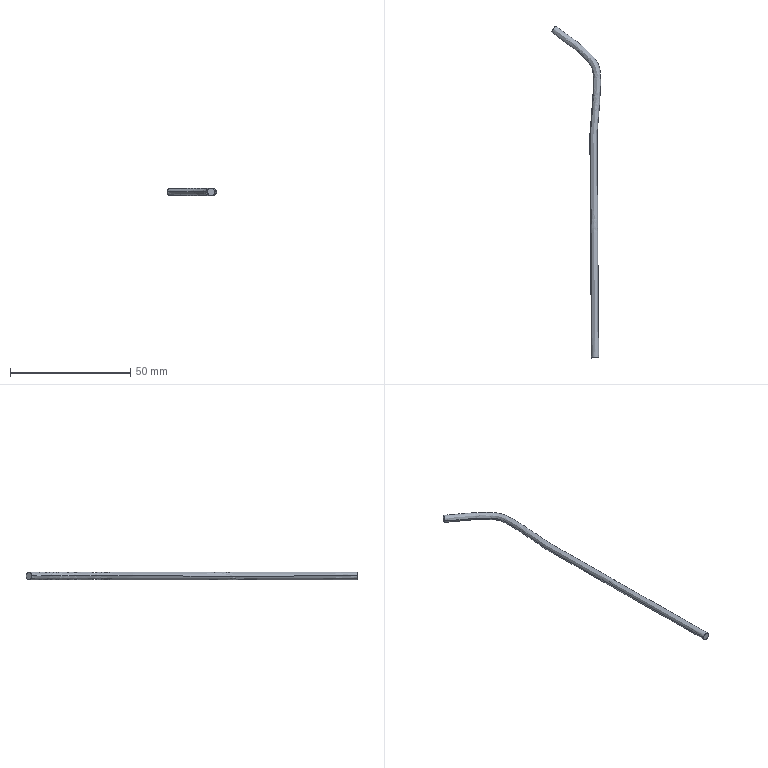Part | NX | features BREP 1 | 1 solid | 4 faces | box 20.548 x 138.141 x 3 mm | volume 1002 mm3 | plane 2 | spline 2
STEP:
#1=CARTESIAN_POINT('',(61.593,-31.891,217.465));
#2=VERTEX_POINT('',#1);
#3=CARTESIAN_POINT('',(64.593,-31.865,217.465));
#4=VERTEX_POINT('',#3);
#5=CARTESIAN_POINT('',(61.593,-31.891,217.465));
#6=CARTESIAN_POINT('',(61.593,-31.891,217.819));
#7=CARTESIAN_POINT('',(61.861,-31.889,218.592));
#8=CARTESIAN_POINT('',(63.093,-31.878,219.152));
#9=CARTESIAN_POINT('',(64.325,-31.867,218.592));
#10=CARTESIAN_POINT('',(64.593,-31.865,217.819));
#11=CARTESIAN_POINT('',(64.593,-31.865,217.465));
#12=B_SPLINE_CURVE_WITH_KNOTS('',3,(#5,#6,#7,#8,#9,#10,#11),.UNSPECIFIED.,.F.,.F.,(4,1,1,1,4),(0.,0.25,0.5,0.75,1.),.UNSPECIFIED.);
#13=EDGE_CURVE('',#2,#4,#12,.T.);
#14=ORIENTED_EDGE('',*,*,#13,.F.);
#15=CARTESIAN_POINT('',(64.593,-31.865,217.465));
#16=CARTESIAN_POINT('',(64.593,-31.865,217.111));
#17=CARTESIAN_POINT('',(64.325,-31.867,216.338));
#18=CARTESIAN_POINT('',(63.093,-31.878,215.778));
#19=CARTESIAN_POINT('',(61.861,-31.889,216.338));
#20=CARTESIAN_POINT('',(61.593,-31.891,217.111));
#21=CARTESIAN_POINT('',(61.593,-31.891,217.465));
#22=B_SPLINE_CURVE_WITH_KNOTS('',3,(#15,#16,#17,#18,#19,#20,#21),.UNSPECIFIED.,.F.,.F.,(4,1,1,1,4),(0.,0.25,0.5,0.75,1.),.QUASI_UNIFORM_KNOTS.);
#23=EDGE_CURVE('',#4,#2,#22,.T.);
#24=ORIENTED_EDGE('',*,*,#23,.F.);
#25=EDGE_LOOP('',(#14,#24));
#26=FACE_BOUND('',#25,.T.);
#27=CARTESIAN_POINT('',(61.593,-31.891,217.465));
#28=DIRECTION('',(0.008906,-1.,0.000000006));
#29=DIRECTION('',(0.,0.000000006,1.));
#30=AXIS2_PLACEMENT_3D('',#27,#28,#29);
#31=PLANE('',#30);
#32=ADVANCED_FACE('',(#26),#31,.T.);
#33=CARTESIAN_POINT('',(44.894,103.809,217.465));
#34=VERTEX_POINT('',#33);
#35=CARTESIAN_POINT('',(44.894,103.809,217.465));
#36=CARTESIAN_POINT('',(46.116,102.935,217.465));
#37=CARTESIAN_POINT('',(48.783,100.951,217.465));
#38=CARTESIAN_POINT('',(52.514,98.365,217.465));
#39=CARTESIAN_POINT('',(55.95,95.618,217.465));
#40=CARTESIAN_POINT('',(58.626,93.056,217.465));
#41=CARTESIAN_POINT('',(60.651,90.876,217.465));
#42=CARTESIAN_POINT('',(61.601,89.557,217.465));
#43=CARTESIAN_POINT('',(61.978,88.512,217.465));
#44=CARTESIAN_POINT('',(62.247,87.211,217.465));
#45=CARTESIAN_POINT('',(62.413,85.422,217.465));
#46=CARTESIAN_POINT('',(62.458,83.217,217.465));
#47=CARTESIAN_POINT('',(62.394,80.239,217.465));
#48=CARTESIAN_POINT('',(62.18,76.415,217.465));
#49=CARTESIAN_POINT('',(61.919,72.728,217.465));
#50=CARTESIAN_POINT('',(61.677,69.609,217.465));
#51=CARTESIAN_POINT('',(61.506,67.528,217.465));
#52=CARTESIAN_POINT('',(61.373,66.009,217.465));
#53=CARTESIAN_POINT('',(61.249,64.63,217.465));
#54=CARTESIAN_POINT('',(61.139,63.519,217.465));
#55=CARTESIAN_POINT('',(61.066,62.809,217.465));
#56=CARTESIAN_POINT('',(60.906,61.459,217.465));
#57=CARTESIAN_POINT('',(60.942,60.335,217.465));
#58=CARTESIAN_POINT('',(60.935,58.917,217.465));
#59=CARTESIAN_POINT('',(60.945,58.217,217.465));
#60=CARTESIAN_POINT('',(60.956,56.671,217.465));
#61=CARTESIAN_POINT('',(60.969,55.141,217.465));
#62=CARTESIAN_POINT('',(60.987,53.132,217.465));
#63=CARTESIAN_POINT('',(61.019,49.703,217.465));
#64=CARTESIAN_POINT('',(61.062,44.953,217.465));
#65=CARTESIAN_POINT('',(61.109,39.145,217.465));
#66=CARTESIAN_POINT('',(61.145,34.01,217.465));
#67=CARTESIAN_POINT('',(61.182,27.92,217.465));
#68=CARTESIAN_POINT('',(61.224,20.363,217.465));
#69=CARTESIAN_POINT('',(61.274,12.258,217.465));
#70=CARTESIAN_POINT('',(61.333,4.336,217.465));
#71=CARTESIAN_POINT('',(61.401,-4.1,217.465));
#72=CARTESIAN_POINT('',(61.473,-13.387,217.465));
#73=CARTESIAN_POINT('',(61.529,-22.629,217.465));
#74=CARTESIAN_POINT('',(61.566,-28.804,217.465));
#75=CARTESIAN_POINT('',(61.593,-31.891,217.465));
#76=B_SPLINE_CURVE_WITH_KNOTS('',3,(#35,#36,#37,#38,#39,#40,#41,#42,#43,#44,#45,#46,#47,#48,#49,#50,#51,#52,#53,#54,#55,#56,#57,#58,#59,#60,#61,#62,#63,#64,#65,#66,#67,#68,#69,#70,#71,#72,#73,#74,#75),.UNSPECIFIED.,.F.,.F.,(4,1,1,1,1,1,1,1,1,1,1,1,1,1,1,1,1,1,1,1,1,1,1,1,1,1,1,1,1,1,1,1,1,1,1,1,1,1,4),(0.,0.03125,0.0625,0.09375,0.125,0.1406,0.1562,0.1641,0.1719,0.1875,0.2031,0.2188,0.25,0.2812,0.2969,0.3125,0.3281,0.3438,0.3477,0.3516,0.3594,0.3672,0.375,0.3906,0.3984,0.4062,0.4219,0.4375,0.4688,0.5,0.5312,0.5625,0.625,0.6875,0.75,0.8125,0.875,0.9375,1.),.UNSPECIFIED.);
#77=EDGE_CURVE('',#34,#2,#76,.T.);
#78=ORIENTED_EDGE('',*,*,#77,.T.);
#79=ORIENTED_EDGE('',*,*,#13,.T.);
#80=CARTESIAN_POINT('',(46.638,106.249,217.465));
#81=VERTEX_POINT('',#80);
#82=CARTESIAN_POINT('',(64.593,-31.865,217.465));
#83=CARTESIAN_POINT('',(64.565,-28.783,217.465));
#84=CARTESIAN_POINT('',(64.529,-22.614,217.465));
#85=CARTESIAN_POINT('',(64.473,-13.365,217.465));
#86=CARTESIAN_POINT('',(64.401,-4.075,217.465));
#87=CARTESIAN_POINT('',(64.333,4.36,217.465));
#88=CARTESIAN_POINT('',(64.274,12.277,217.465));
#89=CARTESIAN_POINT('',(64.224,20.379,217.465));
#90=CARTESIAN_POINT('',(64.182,27.937,217.465));
#91=CARTESIAN_POINT('',(64.145,34.03,217.465));
#92=CARTESIAN_POINT('',(64.109,39.166,217.465));
#93=CARTESIAN_POINT('',(64.062,44.977,217.465));
#94=CARTESIAN_POINT('',(64.019,49.728,217.465));
#95=CARTESIAN_POINT('',(63.987,53.159,217.465));
#96=CARTESIAN_POINT('',(63.968,55.168,217.465));
#97=CARTESIAN_POINT('',(63.956,56.695,217.465));
#98=CARTESIAN_POINT('',(63.944,58.236,217.465));
#99=CARTESIAN_POINT('',(63.939,58.934,217.465));
#100=CARTESIAN_POINT('',(63.935,60.159,217.465));
#101=CARTESIAN_POINT('',(63.935,60.903,217.465));
#102=CARTESIAN_POINT('',(63.94,61.42,217.465));
#103=CARTESIAN_POINT('',(63.949,61.631,217.465));
#104=CARTESIAN_POINT('',(63.977,61.879,217.465));
#105=CARTESIAN_POINT('',(64.028,62.324,217.465));
#106=CARTESIAN_POINT('',(64.074,62.744,217.465));
#107=CARTESIAN_POINT('',(64.124,63.223,217.465));
#108=CARTESIAN_POINT('',(64.198,63.97,217.465));
#109=CARTESIAN_POINT('',(64.277,64.818,217.465));
#110=CARTESIAN_POINT('',(64.383,65.993,217.465));
#111=CARTESIAN_POINT('',(64.495,67.275,217.465));
#112=CARTESIAN_POINT('',(64.667,69.371,217.465));
#113=CARTESIAN_POINT('',(64.91,72.507,217.465));
#114=CARTESIAN_POINT('',(65.173,76.219,217.465));
#115=CARTESIAN_POINT('',(65.393,80.1,217.465));
#116=CARTESIAN_POINT('',(65.457,83.207,217.465));
#117=CARTESIAN_POINT('',(65.414,85.566,217.465));
#118=CARTESIAN_POINT('',(65.224,87.598,217.465));
#119=CARTESIAN_POINT('',(64.899,89.256,217.465));
#120=CARTESIAN_POINT('',(64.241,91.075,217.465));
#121=CARTESIAN_POINT('',(62.896,92.872,217.465));
#122=CARTESIAN_POINT('',(61.283,94.603,217.465));
#123=CARTESIAN_POINT('',(59.649,96.225,217.465));
#124=CARTESIAN_POINT('',(57.318,98.371,217.465));
#125=CARTESIAN_POINT('',(54.277,100.792,217.465));
#126=CARTESIAN_POINT('',(50.495,103.415,217.465));
#127=CARTESIAN_POINT('',(47.924,105.33,217.465));
#128=CARTESIAN_POINT('',(46.638,106.249,217.465));
#129=B_SPLINE_CURVE_WITH_KNOTS('',3,(#82,#83,#84,#85,#86,#87,#88,#89,#90,#91,#92,#93,#94,#95,#96,#97,#98,#99,#100,#101,#102,#103,#104,#105,#106,#107,#108,#109,#110,#111,#112,#113,#114,#115,#116,#117,#118,#119,#120,#121,#122,#123,#124,#125,#126,#127,#128),.UNSPECIFIED.,.F.,.F.,(4,1,1,1,1,1,1,1,1,1,1,1,1,1,1,1,1,1,1,1,1,1,1,1,1,1,1,1,1,1,1,1,1,1,1,1,1,1,1,1,1,1,1,1,4),(0.,0.0625,0.125,0.1875,0.25,0.3125,0.375,0.4375,0.4688,0.5,0.5312,0.5625,0.5781,0.5938,0.6016,0.6094,0.625,0.6328,0.6367,0.6406,0.6426,0.6445,0.6465,0.6484,0.6523,0.6562,0.6641,0.6719,0.6875,0.7031,0.7188,0.75,0.7812,0.7969,0.8125,0.8281,0.8359,0.8438,0.8594,0.875,0.8906,0.9062,0.9375,0.9688,1.),.UNSPECIFIED.);
#130=EDGE_CURVE('',#81,#4,#129,.F.);
#131=ORIENTED_EDGE('',*,*,#130,.F.);
#132=CARTESIAN_POINT('',(44.894,103.809,217.465));
#133=CARTESIAN_POINT('',(44.894,103.809,217.819));
#134=CARTESIAN_POINT('',(45.05,104.027,218.592));
#135=CARTESIAN_POINT('',(45.766,105.029,219.152));
#136=CARTESIAN_POINT('',(46.482,106.031,218.592));
#137=CARTESIAN_POINT('',(46.638,106.249,217.819));
#138=CARTESIAN_POINT('',(46.638,106.249,217.465));
#139=B_SPLINE_CURVE_WITH_KNOTS('',3,(#132,#133,#134,#135,#136,#137,#138),.UNSPECIFIED.,.F.,.F.,(4,1,1,1,4),(0.,0.25,0.5,0.75,1.),.UNSPECIFIED.);
#140=EDGE_CURVE('',#34,#81,#139,.T.);
#141=ORIENTED_EDGE('',*,*,#140,.F.);
#142=EDGE_LOOP('',(#78,#79,#131,#141));
#143=FACE_BOUND('',#142,.T.);
#144=CARTESIAN_POINT('',(64.593,-31.865,217.465));
#145=CARTESIAN_POINT('',(64.593,-31.865,217.819));
#146=CARTESIAN_POINT('',(64.325,-31.867,218.592));
#147=CARTESIAN_POINT('',(63.093,-31.878,219.152));
#148=CARTESIAN_POINT('',(61.861,-31.889,218.592));
#149=CARTESIAN_POINT('',(61.593,-31.891,217.819));
#150=CARTESIAN_POINT('',(61.593,-31.891,217.465));
#151=CARTESIAN_POINT('',(64.563,-28.51,217.465));
#152=CARTESIAN_POINT('',(64.563,-28.51,217.819));
#153=CARTESIAN_POINT('',(64.295,-28.512,218.592));
#154=CARTESIAN_POINT('',(63.063,-28.52,219.152));
#155=CARTESIAN_POINT('',(61.831,-28.529,218.592));
#156=CARTESIAN_POINT('',(61.563,-28.53,217.819));
#157=CARTESIAN_POINT('',(61.563,-28.53,217.465));
#158=CARTESIAN_POINT('',(64.534,-23.475,217.465));
#159=CARTESIAN_POINT('',(64.534,-23.475,217.819));
#160=CARTESIAN_POINT('',(64.266,-23.477,218.592));
#161=CARTESIAN_POINT('',(63.034,-23.483,219.152));
#162=CARTESIAN_POINT('',(61.802,-23.49,218.592));
#163=CARTESIAN_POINT('',(61.534,-23.491,217.819));
#164=CARTESIAN_POINT('',(61.534,-23.491,217.465));
#165=CARTESIAN_POINT('',(64.494,-16.759,217.465));
#166=CARTESIAN_POINT('',(64.494,-16.759,217.819));
#167=CARTESIAN_POINT('',(64.226,-16.76,218.592));
#168=CARTESIAN_POINT('',(62.994,-16.768,219.152));
#169=CARTESIAN_POINT('',(61.762,-16.776,218.592));
#170=CARTESIAN_POINT('',(61.494,-16.778,217.819));
#171=CARTESIAN_POINT('',(61.494,-16.778,217.465));
#172=CARTESIAN_POINT('',(64.458,-11.449,217.465));
#173=CARTESIAN_POINT('',(64.458,-11.449,217.819));
#174=CARTESIAN_POINT('',(64.189,-11.451,218.592));
#175=CARTESIAN_POINT('',(62.958,-11.46,219.152));
#176=CARTESIAN_POINT('',(61.726,-11.469,218.592));
#177=CARTESIAN_POINT('',(61.458,-11.471,217.819));
#178=CARTESIAN_POINT('',(61.458,-11.471,217.465));
#179=CARTESIAN_POINT('',(64.415,-5.882,217.465));
#180=CARTESIAN_POINT('',(64.415,-5.882,217.819));
#181=CARTESIAN_POINT('',(64.147,-5.884,218.592));
#182=CARTESIAN_POINT('',(62.915,-5.894,219.152));
#183=CARTESIAN_POINT('',(61.683,-5.904,218.592));
#184=CARTESIAN_POINT('',(61.415,-5.906,217.819));
#185=CARTESIAN_POINT('',(61.415,-5.906,217.465));
#186=CARTESIAN_POINT('',(64.356,1.522,217.465));
#187=CARTESIAN_POINT('',(64.356,1.522,217.819));
#188=CARTESIAN_POINT('',(64.087,1.52,218.592));
#189=CARTESIAN_POINT('',(62.856,1.51,219.152));
#190=CARTESIAN_POINT('',(61.624,1.5,218.592));
#191=CARTESIAN_POINT('',(61.356,1.498,217.819));
#192=CARTESIAN_POINT('',(61.356,1.498,217.465));
#193=CARTESIAN_POINT('',(64.289,9.937,217.465));
#194=CARTESIAN_POINT('',(64.289,9.937,217.819));
#195=CARTESIAN_POINT('',(64.021,9.936,218.592));
#196=CARTESIAN_POINT('',(62.789,9.927,219.152));
#197=CARTESIAN_POINT('',(61.557,9.918,218.592));
#198=CARTESIAN_POINT('',(61.289,9.917,217.819));
#199=CARTESIAN_POINT('',(61.289,9.917,217.465));
#200=CARTESIAN_POINT('',(64.236,18.351,217.465));
#201=CARTESIAN_POINT('',(64.236,18.351,217.819));
#202=CARTESIAN_POINT('',(63.968,18.35,218.592));
#203=CARTESIAN_POINT('',(62.736,18.343,219.152));
#204=CARTESIAN_POINT('',(61.504,18.336,218.592));
#205=CARTESIAN_POINT('',(61.236,18.334,217.819));
#206=CARTESIAN_POINT('',(61.236,18.334,217.465));
#207=CARTESIAN_POINT('',(64.194,25.757,217.465));
#208=CARTESIAN_POINT('',(64.194,25.757,217.819));
#209=CARTESIAN_POINT('',(63.926,25.756,218.592));
#210=CARTESIAN_POINT('',(62.694,25.749,219.152));
#211=CARTESIAN_POINT('',(61.462,25.742,218.592));
#212=CARTESIAN_POINT('',(61.194,25.741,217.819));
#213=CARTESIAN_POINT('',(61.194,25.741,217.465));
#214=CARTESIAN_POINT('',(64.166,30.569,217.465));
#215=CARTESIAN_POINT('',(64.166,30.569,217.819));
#216=CARTESIAN_POINT('',(63.898,30.568,218.592));
#217=CARTESIAN_POINT('',(62.666,30.56,219.152));
#218=CARTESIAN_POINT('',(61.435,30.553,218.592));
#219=CARTESIAN_POINT('',(61.167,30.552,217.819));
#220=CARTESIAN_POINT('',(61.167,30.552,217.465));
#221=CARTESIAN_POINT('',(64.142,34.39,217.465));
#222=CARTESIAN_POINT('',(64.142,34.39,217.819));
#223=CARTESIAN_POINT('',(63.874,34.388,218.592));
#224=CARTESIAN_POINT('',(62.642,34.38,219.152));
#225=CARTESIAN_POINT('',(61.411,34.372,218.592));
#226=CARTESIAN_POINT('',(61.142,34.371,217.819));
#227=CARTESIAN_POINT('',(61.142,34.371,217.465));
#228=CARTESIAN_POINT('',(64.114,38.442,217.465));
#229=CARTESIAN_POINT('',(64.114,38.442,217.819));
#230=CARTESIAN_POINT('',(63.846,38.44,218.592));
#231=CARTESIAN_POINT('',(62.614,38.431,219.152));
#232=CARTESIAN_POINT('',(61.383,38.422,218.592));
#233=CARTESIAN_POINT('',(61.114,38.42,217.819));
#234=CARTESIAN_POINT('',(61.114,38.42,217.465));
#235=CARTESIAN_POINT('',(64.069,44.22,217.465));
#236=CARTESIAN_POINT('',(64.069,44.22,217.819));
#237=CARTESIAN_POINT('',(63.801,44.218,218.592));
#238=CARTESIAN_POINT('',(62.569,44.209,219.152));
#239=CARTESIAN_POINT('',(61.337,44.199,218.592));
#240=CARTESIAN_POINT('',(61.069,44.197,217.819));
#241=CARTESIAN_POINT('',(61.069,44.197,217.465));
#242=CARTESIAN_POINT('',(64.006,51.151,217.465));
#243=CARTESIAN_POINT('',(64.006,51.151,217.819));
#244=CARTESIAN_POINT('',(63.738,51.149,218.592));
#245=CARTESIAN_POINT('',(62.506,51.138,219.152));
#246=CARTESIAN_POINT('',(61.275,51.127,218.592));
#247=CARTESIAN_POINT('',(61.006,51.125,217.819));
#248=CARTESIAN_POINT('',(61.006,51.125,217.465));
#249=CARTESIAN_POINT('',(63.965,55.427,217.465));
#250=CARTESIAN_POINT('',(63.965,55.427,217.819));
#251=CARTESIAN_POINT('',(63.697,55.425,218.592));
#252=CARTESIAN_POINT('',(62.465,55.413,219.152));
#253=CARTESIAN_POINT('',(61.233,55.401,218.592));
#254=CARTESIAN_POINT('',(60.965,55.398,217.819));
#255=CARTESIAN_POINT('',(60.965,55.398,217.465));
#256=CARTESIAN_POINT('',(63.946,57.988,217.465));
#257=CARTESIAN_POINT('',(63.946,57.988,217.819));
#258=CARTESIAN_POINT('',(63.678,57.986,218.592));
#259=CARTESIAN_POINT('',(62.446,57.978,219.152));
#260=CARTESIAN_POINT('',(61.214,57.969,218.592));
#261=CARTESIAN_POINT('',(60.946,57.968,217.819));
#262=CARTESIAN_POINT('',(60.946,57.968,217.465));
#263=CARTESIAN_POINT('',(63.941,58.709,217.465));
#264=CARTESIAN_POINT('',(63.941,58.709,217.819));
#265=CARTESIAN_POINT('',(63.673,58.708,218.592));
#266=CARTESIAN_POINT('',(62.441,58.702,219.152));
#267=CARTESIAN_POINT('',(61.21,58.696,218.592));
#268=CARTESIAN_POINT('',(60.941,58.694,217.819));
#269=CARTESIAN_POINT('',(60.941,58.694,217.465));
#270=CARTESIAN_POINT('',(63.937,59.434,217.465));
#271=CARTESIAN_POINT('',(63.937,59.434,217.819));
#272=CARTESIAN_POINT('',(63.669,59.433,218.592));
#273=CARTESIAN_POINT('',(62.437,59.429,219.152));
#274=CARTESIAN_POINT('',(61.206,59.425,218.592));
#275=CARTESIAN_POINT('',(60.937,59.424,217.819));
#276=CARTESIAN_POINT('',(60.937,59.424,217.465));
#277=CARTESIAN_POINT('',(63.934,60.323,217.465));
#278=CARTESIAN_POINT('',(63.934,60.323,217.819));
#279=CARTESIAN_POINT('',(63.666,60.322,218.592));
#280=CARTESIAN_POINT('',(62.434,60.317,219.152));
#281=CARTESIAN_POINT('',(61.202,60.312,218.592));
#282=CARTESIAN_POINT('',(60.934,60.311,217.819));
#283=CARTESIAN_POINT('',(60.934,60.311,217.465));
#284=CARTESIAN_POINT('',(63.936,60.979,217.465));
#285=CARTESIAN_POINT('',(63.936,60.979,217.819));
#286=CARTESIAN_POINT('',(63.668,60.981,218.592));
#287=CARTESIAN_POINT('',(62.436,60.99,219.152));
#288=CARTESIAN_POINT('',(61.204,60.999,218.592));
#289=CARTESIAN_POINT('',(60.936,61.001,217.819));
#290=CARTESIAN_POINT('',(60.936,61.001,217.465));
#291=CARTESIAN_POINT('',(63.939,61.327,217.465));
#292=CARTESIAN_POINT('',(63.939,61.327,217.819));
#293=CARTESIAN_POINT('',(63.671,61.329,218.592));
#294=CARTESIAN_POINT('',(62.439,61.34,219.152));
#295=CARTESIAN_POINT('',(61.208,61.35,218.592));
#296=CARTESIAN_POINT('',(60.939,61.353,217.819));
#297=CARTESIAN_POINT('',(60.939,61.353,217.465));
#298=CARTESIAN_POINT('',(63.945,61.554,217.465));
#299=CARTESIAN_POINT('',(63.945,61.554,217.819));
#300=CARTESIAN_POINT('',(63.677,61.565,218.592));
#301=CARTESIAN_POINT('',(62.446,61.616,219.152));
#302=CARTESIAN_POINT('',(61.214,61.667,218.592));
#303=CARTESIAN_POINT('',(60.946,61.678,217.819));
#304=CARTESIAN_POINT('',(60.946,61.678,217.465));
#305=CARTESIAN_POINT('',(63.953,61.659,217.465));
#306=CARTESIAN_POINT('',(63.953,61.659,217.819));
#307=CARTESIAN_POINT('',(63.686,61.687,218.592));
#308=CARTESIAN_POINT('',(62.46,61.816,219.152));
#309=CARTESIAN_POINT('',(61.235,61.944,218.592));
#310=CARTESIAN_POINT('',(60.968,61.972,217.819));
#311=CARTESIAN_POINT('',(60.968,61.972,217.465));
#312=CARTESIAN_POINT('',(63.974,61.85,217.465));
#313=CARTESIAN_POINT('',(63.974,61.85,217.819));
#314=CARTESIAN_POINT('',(63.707,61.881,218.592));
#315=CARTESIAN_POINT('',(62.484,62.025,219.152));
#316=CARTESIAN_POINT('',(61.261,62.169,218.592));
#317=CARTESIAN_POINT('',(60.995,62.201,217.819));
#318=CARTESIAN_POINT('',(60.995,62.201,217.465));
#319=CARTESIAN_POINT('',(64.006,62.133,217.465));
#320=CARTESIAN_POINT('',(64.006,62.133,217.819));
#321=CARTESIAN_POINT('',(63.74,62.164,218.592));
#322=CARTESIAN_POINT('',(62.517,62.304,219.152));
#323=CARTESIAN_POINT('',(61.293,62.445,218.592));
#324=CARTESIAN_POINT('',(61.027,62.476,217.819));
#325=CARTESIAN_POINT('',(61.027,62.476,217.465));
#326=CARTESIAN_POINT('',(64.039,62.423,217.465));
#327=CARTESIAN_POINT('',(64.039,62.423,217.819));
#328=CARTESIAN_POINT('',(63.773,62.452,218.592));
#329=CARTESIAN_POINT('',(62.548,62.587,219.152));
#330=CARTESIAN_POINT('',(61.324,62.721,218.592));
#331=CARTESIAN_POINT('',(61.057,62.751,217.819));
#332=CARTESIAN_POINT('',(61.057,62.751,217.465));
#333=CARTESIAN_POINT('',(64.136,63.316,217.465));
#334=CARTESIAN_POINT('',(64.136,63.316,217.819));
#335=CARTESIAN_POINT('',(63.869,63.342,218.592));
#336=CARTESIAN_POINT('',(62.643,63.463,219.152));
#337=CARTESIAN_POINT('',(61.417,63.584,218.592));
#338=CARTESIAN_POINT('',(61.15,63.611,217.819));
#339=CARTESIAN_POINT('',(61.15,63.611,217.465));
#340=CARTESIAN_POINT('',(64.273,64.758,217.465));
#341=CARTESIAN_POINT('',(64.273,64.758,217.819));
#342=CARTESIAN_POINT('',(64.006,64.782,218.592));
#343=CARTESIAN_POINT('',(62.78,64.896,219.152));
#344=CARTESIAN_POINT('',(61.553,65.009,218.592));
#345=CARTESIAN_POINT('',(61.286,65.033,217.819));
#346=CARTESIAN_POINT('',(61.286,65.033,217.465));
#347=CARTESIAN_POINT('',(64.411,66.305,217.465));
#348=CARTESIAN_POINT('',(64.411,66.305,217.819));
#349=CARTESIAN_POINT('',(64.144,66.329,218.592));
#350=CARTESIAN_POINT('',(62.917,66.438,219.152));
#351=CARTESIAN_POINT('',(61.69,66.547,218.592));
#352=CARTESIAN_POINT('',(61.423,66.57,217.819));
#353=CARTESIAN_POINT('',(61.423,66.57,217.465));
#354=CARTESIAN_POINT('',(64.542,67.839,217.465));
#355=CARTESIAN_POINT('',(64.542,67.839,217.819));
#356=CARTESIAN_POINT('',(64.275,67.861,218.592));
#357=CARTESIAN_POINT('',(63.047,67.963,219.152));
#358=CARTESIAN_POINT('',(61.82,68.066,218.592));
#359=CARTESIAN_POINT('',(61.552,68.088,217.819));
#360=CARTESIAN_POINT('',(61.552,68.088,217.465));
#361=CARTESIAN_POINT('',(64.725,70.094,217.465));
#362=CARTESIAN_POINT('',(64.725,70.094,217.819));
#363=CARTESIAN_POINT('',(64.457,70.115,218.592));
#364=CARTESIAN_POINT('',(63.229,70.211,219.152));
#365=CARTESIAN_POINT('',(62.001,70.307,218.592));
#366=CARTESIAN_POINT('',(61.734,70.328,217.819));
#367=CARTESIAN_POINT('',(61.734,70.328,217.465));
#368=CARTESIAN_POINT('',(64.913,72.564,217.465));
#369=CARTESIAN_POINT('',(64.913,72.564,217.819));
#370=CARTESIAN_POINT('',(64.645,72.584,218.592));
#371=CARTESIAN_POINT('',(63.417,72.674,219.152));
#372=CARTESIAN_POINT('',(62.188,72.765,218.592));
#373=CARTESIAN_POINT('',(61.921,72.784,217.819));
#374=CARTESIAN_POINT('',(61.921,72.784,217.465));
#375=CARTESIAN_POINT('',(65.092,75.101,217.465));
#376=CARTESIAN_POINT('',(65.092,75.101,217.819));
#377=CARTESIAN_POINT('',(64.825,75.119,218.592));
#378=CARTESIAN_POINT('',(63.596,75.202,219.152));
#379=CARTESIAN_POINT('',(62.367,75.285,218.592));
#380=CARTESIAN_POINT('',(62.099,75.304,217.819));
#381=CARTESIAN_POINT('',(62.099,75.304,217.465));
#382=CARTESIAN_POINT('',(65.254,77.651,217.465));
#383=CARTESIAN_POINT('',(65.254,77.651,217.819));
#384=CARTESIAN_POINT('',(64.986,77.666,218.592));
#385=CARTESIAN_POINT('',(63.757,77.738,219.152));
#386=CARTESIAN_POINT('',(62.527,77.81,218.592));
#387=CARTESIAN_POINT('',(62.259,77.826,217.819));
#388=CARTESIAN_POINT('',(62.259,77.826,217.465));
#389=CARTESIAN_POINT('',(65.37,79.919,217.465));
#390=CARTESIAN_POINT('',(65.37,79.919,217.819));
#391=CARTESIAN_POINT('',(65.102,79.931,218.592));
#392=CARTESIAN_POINT('',(63.871,79.985,219.152));
#393=CARTESIAN_POINT('',(62.641,80.039,218.592));
#394=CARTESIAN_POINT('',(62.373,80.051,217.819));
#395=CARTESIAN_POINT('',(62.373,80.051,217.465));
#396=CARTESIAN_POINT('',(65.432,81.853,217.465));
#397=CARTESIAN_POINT('',(65.432,81.853,217.819));
#398=CARTESIAN_POINT('',(65.164,81.86,218.592));
#399=CARTESIAN_POINT('',(63.932,81.888,219.152));
#400=CARTESIAN_POINT('',(62.701,81.916,218.592));
#401=CARTESIAN_POINT('',(62.433,81.922,217.819));
#402=CARTESIAN_POINT('',(62.433,81.922,217.465));
#403=CARTESIAN_POINT('',(65.455,83.932,217.465));
#404=CARTESIAN_POINT('',(65.455,83.932,217.819));
#405=CARTESIAN_POINT('',(65.186,83.93,218.592));
#406=CARTESIAN_POINT('',(63.955,83.916,219.152));
#407=CARTESIAN_POINT('',(62.723,83.903,218.592));
#408=CARTESIAN_POINT('',(62.455,83.9,217.819));
#409=CARTESIAN_POINT('',(62.455,83.9,217.465));
#410=CARTESIAN_POINT('',(65.396,85.962,217.465));
#411=CARTESIAN_POINT('',(65.396,85.962,217.819));
#412=CARTESIAN_POINT('',(65.127,85.946,218.592));
#413=CARTESIAN_POINT('',(63.895,85.874,219.152));
#414=CARTESIAN_POINT('',(62.663,85.802,218.592));
#415=CARTESIAN_POINT('',(62.394,85.786,217.819));
#416=CARTESIAN_POINT('',(62.394,85.786,217.465));
#417=CARTESIAN_POINT('',(65.156,87.943,217.465));
#418=CARTESIAN_POINT('',(65.156,87.943,217.819));
#419=CARTESIAN_POINT('',(64.891,87.902,218.592));
#420=CARTESIAN_POINT('',(63.674,87.713,219.152));
#421=CARTESIAN_POINT('',(62.456,87.523,218.592));
#422=CARTESIAN_POINT('',(62.191,87.482,217.819));
#423=CARTESIAN_POINT('',(62.191,87.482,217.465));
#424=CARTESIAN_POINT('',(64.928,89.112,217.465));
#425=CARTESIAN_POINT('',(64.928,89.112,217.819));
#426=CARTESIAN_POINT('',(64.666,89.048,218.592));
#427=CARTESIAN_POINT('',(63.465,88.757,219.152));
#428=CARTESIAN_POINT('',(62.265,88.465,218.592));
#429=CARTESIAN_POINT('',(62.003,88.401,217.819));
#430=CARTESIAN_POINT('',(62.003,88.401,217.465));
#431=CARTESIAN_POINT('',(64.568,90.195,217.465));
#432=CARTESIAN_POINT('',(64.568,90.195,217.819));
#433=CARTESIAN_POINT('',(64.319,90.093,218.592));
#434=CARTESIAN_POINT('',(63.175,89.627,219.152));
#435=CARTESIAN_POINT('',(62.031,89.162,218.592));
#436=CARTESIAN_POINT('',(61.782,89.06,217.819));
#437=CARTESIAN_POINT('',(61.782,89.06,217.465));
#438=CARTESIAN_POINT('',(64.047,91.264,217.465));
#439=CARTESIAN_POINT('',(64.047,91.264,217.819));
#440=CARTESIAN_POINT('',(63.816,91.124,218.592));
#441=CARTESIAN_POINT('',(62.759,90.482,219.152));
#442=CARTESIAN_POINT('',(61.701,89.84,218.592));
#443=CARTESIAN_POINT('',(61.471,89.7,217.819));
#444=CARTESIAN_POINT('',(61.471,89.7,217.465));
#445=CARTESIAN_POINT('',(63.274,92.372,217.465));
#446=CARTESIAN_POINT('',(63.274,92.372,217.819));
#447=CARTESIAN_POINT('',(63.064,92.205,218.592));
#448=CARTESIAN_POINT('',(62.098,91.437,219.152));
#449=CARTESIAN_POINT('',(61.133,90.669,218.592));
#450=CARTESIAN_POINT('',(60.922,90.502,217.819));
#451=CARTESIAN_POINT('',(60.922,90.502,217.465));
#452=CARTESIAN_POINT('',(62.058,93.788,217.465));
#453=CARTESIAN_POINT('',(62.058,93.788,217.819));
#454=CARTESIAN_POINT('',(61.862,93.604,218.592));
#455=CARTESIAN_POINT('',(60.961,92.763,219.152));
#456=CARTESIAN_POINT('',(60.061,91.921,218.592));
#457=CARTESIAN_POINT('',(59.865,91.738,217.819));
#458=CARTESIAN_POINT('',(59.865,91.738,217.465));
#459=CARTESIAN_POINT('',(60.605,95.291,217.465));
#460=CARTESIAN_POINT('',(60.605,95.291,217.819));
#461=CARTESIAN_POINT('',(60.415,95.102,218.592));
#462=CARTESIAN_POINT('',(59.543,94.231,219.152));
#463=CARTESIAN_POINT('',(58.672,93.361,218.592));
#464=CARTESIAN_POINT('',(58.482,93.171,217.819));
#465=CARTESIAN_POINT('',(58.482,93.171,217.465));
#466=CARTESIAN_POINT('',(58.887,96.945,217.465));
#467=CARTESIAN_POINT('',(58.887,96.945,217.819));
#468=CARTESIAN_POINT('',(58.705,96.748,218.592));
#469=CARTESIAN_POINT('',(57.869,95.843,219.152));
#470=CARTESIAN_POINT('',(57.033,94.937,218.592));
#471=CARTESIAN_POINT('',(56.851,94.74,217.819));
#472=CARTESIAN_POINT('',(56.851,94.74,217.465));
#473=CARTESIAN_POINT('',(57.119,98.505,217.465));
#474=CARTESIAN_POINT('',(57.119,98.505,217.819));
#475=CARTESIAN_POINT('',(56.946,98.3,218.592));
#476=CARTESIAN_POINT('',(56.151,97.359,219.152));
#477=CARTESIAN_POINT('',(55.356,96.418,218.592));
#478=CARTESIAN_POINT('',(55.183,96.213,217.819));
#479=CARTESIAN_POINT('',(55.183,96.213,217.465));
#480=CARTESIAN_POINT('',(54.83,100.355,217.465));
#481=CARTESIAN_POINT('',(54.83,100.355,217.819));
#482=CARTESIAN_POINT('',(54.669,100.141,218.592));
#483=CARTESIAN_POINT('',(53.928,99.155,219.152));
#484=CARTESIAN_POINT('',(53.188,98.17,218.592));
#485=CARTESIAN_POINT('',(53.027,97.956,217.819));
#486=CARTESIAN_POINT('',(53.027,97.956,217.465));
#487=CARTESIAN_POINT('',(52.61,101.945,217.465));
#488=CARTESIAN_POINT('',(52.61,101.945,217.819));
#489=CARTESIAN_POINT('',(52.456,101.726,218.592));
#490=CARTESIAN_POINT('',(51.746,100.719,219.152));
#491=CARTESIAN_POINT('',(51.037,99.712,218.592));
#492=CARTESIAN_POINT('',(50.882,99.493,217.819));
#493=CARTESIAN_POINT('',(50.882,99.493,217.465));
#494=CARTESIAN_POINT('',(50.558,103.4,217.465));
#495=CARTESIAN_POINT('',(50.558,103.4,217.819));
#496=CARTESIAN_POINT('',(50.403,103.182,218.592));
#497=CARTESIAN_POINT('',(49.687,102.179,219.152));
#498=CARTESIAN_POINT('',(48.972,101.176,218.592));
#499=CARTESIAN_POINT('',(48.817,100.958,217.819));
#500=CARTESIAN_POINT('',(48.817,100.958,217.465));
#501=CARTESIAN_POINT('',(48.797,104.666,217.465));
#502=CARTESIAN_POINT('',(48.797,104.666,217.819));
#503=CARTESIAN_POINT('',(48.639,104.45,218.592));
#504=CARTESIAN_POINT('',(47.913,103.456,219.152));
#505=CARTESIAN_POINT('',(47.186,102.461,218.592));
#506=CARTESIAN_POINT('',(47.028,102.245,217.819));
#507=CARTESIAN_POINT('',(47.028,102.245,217.465));
#508=CARTESIAN_POINT('',(47.511,105.625,217.465));
#509=CARTESIAN_POINT('',(47.511,105.625,217.819));
#510=CARTESIAN_POINT('',(47.351,105.41,218.592));
#511=CARTESIAN_POINT('',(46.617,104.42,219.152));
#512=CARTESIAN_POINT('',(45.883,103.431,218.592));
#513=CARTESIAN_POINT('',(45.724,103.216,217.819));
#514=CARTESIAN_POINT('',(45.724,103.216,217.465));
#515=CARTESIAN_POINT('',(46.638,106.249,217.465));
#516=CARTESIAN_POINT('',(46.638,106.249,217.819));
#517=CARTESIAN_POINT('',(46.482,106.031,218.592));
#518=CARTESIAN_POINT('',(45.766,105.029,219.152));
#519=CARTESIAN_POINT('',(45.05,104.027,218.592));
#520=CARTESIAN_POINT('',(44.894,103.809,217.819));
#521=CARTESIAN_POINT('',(44.894,103.809,217.465));
#522=B_SPLINE_SURFACE_WITH_KNOTS('',3,3,((#144,#145,#146,#147,#148,#149,#150),(#151,#152,#153,#154,#155,#156,#157),(#158,#159,#160,#161,#162,#163,#164),(#165,#166,#167,#168,#169,#170,#171),(#172,#173,#174,#175,#176,#177,#178),(#179,#180,#181,#182,#183,#184,#185),(#186,#187,#188,#189,#190,#191,#192),(#193,#194,#195,#196,#197,#198,#199),(#200,#201,#202,#203,#204,#205,#206),(#207,#208,#209,#210,#211,#212,#213),(#214,#215,#216,#217,#218,#219,#220),(#221,#222,#223,#224,#225,#226,#227),(#228,#229,#230,#231,#232,#233,#234),(#235,#236,#237,#238,#239,#240,#241),(#242,#243,#244,#245,#246,#247,#248),(#249,#250,#251,#252,#253,#254,#255),(#256,#257,#258,#259,#260,#261,#262),(#263,#264,#265,#266,#267,#268,#269),(#270,#271,#272,#273,#274,#275,#276),(#277,#278,#279,#280,#281,#282,#283),(#284,#285,#286,#287,#288,#289,#290),(#291,#292,#293,#294,#295,#296,#297),(#298,#299,#300,#301,#302,#303,#304),(#305,#306,#307,#308,#309,#310,#311),(#312,#313,#314,#315,#316,#317,#318),(#319,#320,#321,#322,#323,#324,#325),(#326,#327,#328,#329,#330,#331,#332),(#333,#334,#335,#336,#337,#338,#339),(#340,#341,#342,#343,#344,#345,#346),(#347,#348,#349,#350,#351,#352,#353),(#354,#355,#356,#357,#358,#359,#360),(#361,#362,#363,#364,#365,#366,#367),(#368,#369,#370,#371,#372,#373,#374),(#375,#376,#377,#378,#379,#380,#381),(#382,#383,#384,#385,#386,#387,#388),(#389,#390,#391,#392,#393,#394,#395),(#396,#397,#398,#399,#400,#401,#402),(#403,#404,#405,#406,#407,#408,#409),(#410,#411,#412,#413,#414,#415,#416),(#417,#418,#419,#420,#421,#422,#423),(#424,#425,#426,#427,#428,#429,#430),(#431,#432,#433,#434,#435,#436,#437),(#438,#439,#440,#441,#442,#443,#444),(#445,#446,#447,#448,#449,#450,#451),(#452,#453,#454,#455,#456,#457,#458),(#459,#460,#461,#462,#463,#464,#465),(#466,#467,#468,#469,#470,#471,#472),(#473,#474,#475,#476,#477,#478,#479),(#480,#481,#482,#483,#484,#485,#486),(#487,#488,#489,#490,#491,#492,#493),(#494,#495,#496,#497,#498,#499,#500),(#501,#502,#503,#504,#505,#506,#507),(#508,#509,#510,#511,#512,#513,#514),(#515,#516,#517,#518,#519,#520,#521)),.UNSPECIFIED.,.F.,.F.,.F.,(4,1,1,1,1,1,1,1,1,1,1,1,1,1,1,1,1,1,1,1,1,1,1,1,1,1,1,1,1,1,1,1,1,1,1,1,1,1,1,1,1,1,1,1,1,1,1,1,1,1,1,4),(4,1,1,1,4),(0.009495,0.07624,0.1096,0.143,0.1817,0.2204,0.2979,0.3754,0.4141,0.4528,0.4713,0.4898,0.5267,0.5637,0.6006,0.6084,0.6162,0.624,0.6318,0.6346,0.6373,0.6388,0.6402,0.6415,0.6429,0.6443,0.6456,0.66,0.6743,0.6886,0.703,0.7202,0.7375,0.7547,0.772,0.7823,0.7926,0.8132,0.8215,0.8298,0.8349,0.8399,0.849,0.8581,0.8744,0.8906,0.9052,0.9198,0.9489,0.9593,0.9697,0.9905),(0.02123,0.2607,0.5002,0.7396,0.9791),.UNSPECIFIED.);
#523=ADVANCED_FACE('',(#143),#522,.T.);
#524=ORIENTED_EDGE('',*,*,#130,.T.);
#525=ORIENTED_EDGE('',*,*,#23,.T.);
#526=ORIENTED_EDGE('',*,*,#77,.F.);
#527=CARTESIAN_POINT('',(46.638,106.249,217.465));
#528=CARTESIAN_POINT('',(46.638,106.249,217.111));
#529=CARTESIAN_POINT('',(46.482,106.031,216.338));
#530=CARTESIAN_POINT('',(45.766,105.029,215.778));
#531=CARTESIAN_POINT('',(45.05,104.027,216.338));
#532=CARTESIAN_POINT('',(44.894,103.809,217.111));
#533=CARTESIAN_POINT('',(44.894,103.809,217.465));
#534=B_SPLINE_CURVE_WITH_KNOTS('',3,(#527,#528,#529,#530,#531,#532,#533),.UNSPECIFIED.,.F.,.F.,(4,1,1,1,4),(0.,0.25,0.5,0.75,1.),.UNSPECIFIED.);
#535=EDGE_CURVE('',#81,#34,#534,.T.);
#536=ORIENTED_EDGE('',*,*,#535,.F.);
#537=EDGE_LOOP('',(#524,#525,#526,#536));
#538=FACE_BOUND('',#537,.T.);
#539=CARTESIAN_POINT('',(61.593,-31.891,217.465));
#540=CARTESIAN_POINT('',(61.593,-31.891,217.111));
#541=CARTESIAN_POINT('',(61.861,-31.889,216.338));
#542=CARTESIAN_POINT('',(63.093,-31.878,215.778));
#543=CARTESIAN_POINT('',(64.325,-31.867,216.338));
#544=CARTESIAN_POINT('',(64.593,-31.865,217.111));
#545=CARTESIAN_POINT('',(64.593,-31.865,217.465));
#546=CARTESIAN_POINT('',(61.563,-28.53,217.465));
#547=CARTESIAN_POINT('',(61.563,-28.53,217.111));
#548=CARTESIAN_POINT('',(61.831,-28.529,216.338));
#549=CARTESIAN_POINT('',(63.063,-28.52,215.778));
#550=CARTESIAN_POINT('',(64.295,-28.512,216.338));
#551=CARTESIAN_POINT('',(64.563,-28.51,217.111));
#552=CARTESIAN_POINT('',(64.563,-28.51,217.465));
#553=CARTESIAN_POINT('',(61.534,-23.491,217.465));
#554=CARTESIAN_POINT('',(61.534,-23.491,217.111));
#555=CARTESIAN_POINT('',(61.802,-23.49,216.338));
#556=CARTESIAN_POINT('',(63.034,-23.483,215.778));
#557=CARTESIAN_POINT('',(64.266,-23.477,216.338));
#558=CARTESIAN_POINT('',(64.534,-23.475,217.111));
#559=CARTESIAN_POINT('',(64.534,-23.475,217.465));
#560=CARTESIAN_POINT('',(61.494,-16.778,217.465));
#561=CARTESIAN_POINT('',(61.494,-16.778,217.111));
#562=CARTESIAN_POINT('',(61.762,-16.776,216.338));
#563=CARTESIAN_POINT('',(62.994,-16.768,215.778));
#564=CARTESIAN_POINT('',(64.226,-16.76,216.338));
#565=CARTESIAN_POINT('',(64.494,-16.759,217.111));
#566=CARTESIAN_POINT('',(64.494,-16.759,217.465));
#567=CARTESIAN_POINT('',(61.458,-11.471,217.465));
#568=CARTESIAN_POINT('',(61.458,-11.471,217.111));
#569=CARTESIAN_POINT('',(61.726,-11.469,216.338));
#570=CARTESIAN_POINT('',(62.958,-11.46,215.778));
#571=CARTESIAN_POINT('',(64.189,-11.451,216.338));
#572=CARTESIAN_POINT('',(64.458,-11.449,217.111));
#573=CARTESIAN_POINT('',(64.458,-11.449,217.465));
#574=CARTESIAN_POINT('',(61.415,-5.906,217.465));
#575=CARTESIAN_POINT('',(61.415,-5.906,217.111));
#576=CARTESIAN_POINT('',(61.683,-5.904,216.338));
#577=CARTESIAN_POINT('',(62.915,-5.894,215.778));
#578=CARTESIAN_POINT('',(64.147,-5.884,216.338));
#579=CARTESIAN_POINT('',(64.415,-5.882,217.111));
#580=CARTESIAN_POINT('',(64.415,-5.882,217.465));
#581=CARTESIAN_POINT('',(61.356,1.498,217.465));
#582=CARTESIAN_POINT('',(61.356,1.498,217.111));
#583=CARTESIAN_POINT('',(61.624,1.5,216.338));
#584=CARTESIAN_POINT('',(62.856,1.51,215.778));
#585=CARTESIAN_POINT('',(64.087,1.52,216.338));
#586=CARTESIAN_POINT('',(64.356,1.522,217.111));
#587=CARTESIAN_POINT('',(64.356,1.522,217.465));
#588=CARTESIAN_POINT('',(61.289,9.917,217.465));
#589=CARTESIAN_POINT('',(61.289,9.917,217.111));
#590=CARTESIAN_POINT('',(61.557,9.918,216.338));
#591=CARTESIAN_POINT('',(62.789,9.927,215.778));
#592=CARTESIAN_POINT('',(64.021,9.936,216.338));
#593=CARTESIAN_POINT('',(64.289,9.937,217.111));
#594=CARTESIAN_POINT('',(64.289,9.937,217.465));
#595=CARTESIAN_POINT('',(61.236,18.334,217.465));
#596=CARTESIAN_POINT('',(61.236,18.334,217.111));
#597=CARTESIAN_POINT('',(61.504,18.336,216.338));
#598=CARTESIAN_POINT('',(62.736,18.343,215.778));
#599=CARTESIAN_POINT('',(63.968,18.35,216.338));
#600=CARTESIAN_POINT('',(64.236,18.351,217.111));
#601=CARTESIAN_POINT('',(64.236,18.351,217.465));
#602=CARTESIAN_POINT('',(61.194,25.741,217.465));
#603=CARTESIAN_POINT('',(61.194,25.741,217.111));
#604=CARTESIAN_POINT('',(61.462,25.742,216.338));
#605=CARTESIAN_POINT('',(62.694,25.749,215.778));
#606=CARTESIAN_POINT('',(63.926,25.756,216.338));
#607=CARTESIAN_POINT('',(64.194,25.757,217.111));
#608=CARTESIAN_POINT('',(64.194,25.757,217.465));
#609=CARTESIAN_POINT('',(61.167,30.552,217.465));
#610=CARTESIAN_POINT('',(61.167,30.552,217.111));
#611=CARTESIAN_POINT('',(61.435,30.553,216.338));
#612=CARTESIAN_POINT('',(62.666,30.56,215.778));
#613=CARTESIAN_POINT('',(63.898,30.568,216.338));
#614=CARTESIAN_POINT('',(64.166,30.569,217.111));
#615=CARTESIAN_POINT('',(64.166,30.569,217.465));
#616=CARTESIAN_POINT('',(61.142,34.371,217.465));
#617=CARTESIAN_POINT('',(61.142,34.371,217.111));
#618=CARTESIAN_POINT('',(61.411,34.372,216.338));
#619=CARTESIAN_POINT('',(62.642,34.38,215.778));
#620=CARTESIAN_POINT('',(63.874,34.388,216.338));
#621=CARTESIAN_POINT('',(64.142,34.39,217.111));
#622=CARTESIAN_POINT('',(64.142,34.39,217.465));
#623=CARTESIAN_POINT('',(61.114,38.42,217.465));
#624=CARTESIAN_POINT('',(61.114,38.42,217.111));
#625=CARTESIAN_POINT('',(61.383,38.422,216.338));
#626=CARTESIAN_POINT('',(62.614,38.431,215.778));
#627=CARTESIAN_POINT('',(63.846,38.44,216.338));
#628=CARTESIAN_POINT('',(64.114,38.442,217.111));
#629=CARTESIAN_POINT('',(64.114,38.442,217.465));
#630=CARTESIAN_POINT('',(61.069,44.197,217.465));
#631=CARTESIAN_POINT('',(61.069,44.197,217.111));
#632=CARTESIAN_POINT('',(61.337,44.199,216.338));
#633=CARTESIAN_POINT('',(62.569,44.209,215.778));
#634=CARTESIAN_POINT('',(63.801,44.218,216.338));
#635=CARTESIAN_POINT('',(64.069,44.22,217.111));
#636=CARTESIAN_POINT('',(64.069,44.22,217.465));
#637=CARTESIAN_POINT('',(61.006,51.125,217.465));
#638=CARTESIAN_POINT('',(61.006,51.125,217.111));
#639=CARTESIAN_POINT('',(61.275,51.127,216.338));
#640=CARTESIAN_POINT('',(62.506,51.138,215.778));
#641=CARTESIAN_POINT('',(63.738,51.149,216.338));
#642=CARTESIAN_POINT('',(64.006,51.151,217.111));
#643=CARTESIAN_POINT('',(64.006,51.151,217.465));
#644=CARTESIAN_POINT('',(60.965,55.398,217.465));
#645=CARTESIAN_POINT('',(60.965,55.398,217.111));
#646=CARTESIAN_POINT('',(61.233,55.401,216.338));
#647=CARTESIAN_POINT('',(62.465,55.413,215.778));
#648=CARTESIAN_POINT('',(63.697,55.425,216.338));
#649=CARTESIAN_POINT('',(63.965,55.427,217.111));
#650=CARTESIAN_POINT('',(63.965,55.427,217.465));
#651=CARTESIAN_POINT('',(60.946,57.968,217.465));
#652=CARTESIAN_POINT('',(60.946,57.968,217.111));
#653=CARTESIAN_POINT('',(61.214,57.969,216.338));
#654=CARTESIAN_POINT('',(62.446,57.978,215.778));
#655=CARTESIAN_POINT('',(63.678,57.986,216.338));
#656=CARTESIAN_POINT('',(63.946,57.988,217.111));
#657=CARTESIAN_POINT('',(63.946,57.988,217.465));
#658=CARTESIAN_POINT('',(60.941,58.694,217.465));
#659=CARTESIAN_POINT('',(60.941,58.694,217.111));
#660=CARTESIAN_POINT('',(61.21,58.696,216.338));
#661=CARTESIAN_POINT('',(62.441,58.702,215.778));
#662=CARTESIAN_POINT('',(63.673,58.708,216.338));
#663=CARTESIAN_POINT('',(63.941,58.709,217.111));
#664=CARTESIAN_POINT('',(63.941,58.709,217.465));
#665=CARTESIAN_POINT('',(60.937,59.424,217.465));
#666=CARTESIAN_POINT('',(60.937,59.424,217.111));
#667=CARTESIAN_POINT('',(61.206,59.425,216.338));
#668=CARTESIAN_POINT('',(62.437,59.429,215.778));
#669=CARTESIAN_POINT('',(63.669,59.433,216.338));
#670=CARTESIAN_POINT('',(63.937,59.434,217.111));
#671=CARTESIAN_POINT('',(63.937,59.434,217.465));
#672=CARTESIAN_POINT('',(60.934,60.311,217.465));
#673=CARTESIAN_POINT('',(60.934,60.311,217.111));
#674=CARTESIAN_POINT('',(61.202,60.312,216.338));
#675=CARTESIAN_POINT('',(62.434,60.317,215.778));
#676=CARTESIAN_POINT('',(63.666,60.322,216.338));
#677=CARTESIAN_POINT('',(63.934,60.323,217.111));
#678=CARTESIAN_POINT('',(63.934,60.323,217.465));
#679=CARTESIAN_POINT('',(60.936,61.001,217.465));
#680=CARTESIAN_POINT('',(60.936,61.001,217.111));
#681=CARTESIAN_POINT('',(61.204,60.999,216.338));
#682=CARTESIAN_POINT('',(62.436,60.99,215.778));
#683=CARTESIAN_POINT('',(63.668,60.981,216.338));
#684=CARTESIAN_POINT('',(63.936,60.979,217.111));
#685=CARTESIAN_POINT('',(63.936,60.979,217.465));
#686=CARTESIAN_POINT('',(60.939,61.353,217.465));
#687=CARTESIAN_POINT('',(60.939,61.353,217.111));
#688=CARTESIAN_POINT('',(61.208,61.35,216.338));
#689=CARTESIAN_POINT('',(62.439,61.34,215.778));
#690=CARTESIAN_POINT('',(63.671,61.329,216.338));
#691=CARTESIAN_POINT('',(63.939,61.327,217.111));
#692=CARTESIAN_POINT('',(63.939,61.327,217.465));
#693=CARTESIAN_POINT('',(60.946,61.678,217.465));
#694=CARTESIAN_POINT('',(60.946,61.678,217.111));
#695=CARTESIAN_POINT('',(61.214,61.667,216.338));
#696=CARTESIAN_POINT('',(62.446,61.616,215.778));
#697=CARTESIAN_POINT('',(63.677,61.565,216.338));
#698=CARTESIAN_POINT('',(63.945,61.554,217.111));
#699=CARTESIAN_POINT('',(63.945,61.554,217.465));
#700=CARTESIAN_POINT('',(60.968,61.972,217.465));
#701=CARTESIAN_POINT('',(60.968,61.972,217.111));
#702=CARTESIAN_POINT('',(61.235,61.944,216.338));
#703=CARTESIAN_POINT('',(62.46,61.816,215.778));
#704=CARTESIAN_POINT('',(63.686,61.687,216.338));
#705=CARTESIAN_POINT('',(63.953,61.659,217.111));
#706=CARTESIAN_POINT('',(63.953,61.659,217.465));
#707=CARTESIAN_POINT('',(60.995,62.201,217.465));
#708=CARTESIAN_POINT('',(60.995,62.201,217.111));
#709=CARTESIAN_POINT('',(61.261,62.169,216.338));
#710=CARTESIAN_POINT('',(62.484,62.025,215.778));
#711=CARTESIAN_POINT('',(63.707,61.881,216.338));
#712=CARTESIAN_POINT('',(63.974,61.85,217.111));
#713=CARTESIAN_POINT('',(63.974,61.85,217.465));
#714=CARTESIAN_POINT('',(61.027,62.476,217.465));
#715=CARTESIAN_POINT('',(61.027,62.476,217.111));
#716=CARTESIAN_POINT('',(61.293,62.445,216.338));
#717=CARTESIAN_POINT('',(62.517,62.305,215.778));
#718=CARTESIAN_POINT('',(63.74,62.164,216.338));
#719=CARTESIAN_POINT('',(64.007,62.133,217.111));
#720=CARTESIAN_POINT('',(64.007,62.133,217.465));
#721=CARTESIAN_POINT('',(61.057,62.751,217.465));
#722=CARTESIAN_POINT('',(61.057,62.751,217.111));
#723=CARTESIAN_POINT('',(61.324,62.721,216.338));
#724=CARTESIAN_POINT('',(62.548,62.586,215.778));
#725=CARTESIAN_POINT('',(63.773,62.452,216.338));
#726=CARTESIAN_POINT('',(64.039,62.422,217.111));
#727=CARTESIAN_POINT('',(64.039,62.422,217.465));
#728=CARTESIAN_POINT('',(61.082,62.98,217.465));
#729=CARTESIAN_POINT('',(61.082,62.98,217.111));
#730=CARTESIAN_POINT('',(61.349,62.951,216.338));
#731=CARTESIAN_POINT('',(62.574,62.82,215.778));
#732=CARTESIAN_POINT('',(63.798,62.689,216.338));
#733=CARTESIAN_POINT('',(64.065,62.66,217.111));
#734=CARTESIAN_POINT('',(64.065,62.66,217.465));
#735=CARTESIAN_POINT('',(61.108,63.22,217.465));
#736=CARTESIAN_POINT('',(61.108,63.22,217.111));
#737=CARTESIAN_POINT('',(61.374,63.193,216.338));
#738=CARTESIAN_POINT('',(62.6,63.065,215.778));
#739=CARTESIAN_POINT('',(63.825,62.937,216.338));
#740=CARTESIAN_POINT('',(64.091,62.909,217.111));
#741=CARTESIAN_POINT('',(64.091,62.909,217.465));
#742=CARTESIAN_POINT('',(61.144,63.572,217.465));
#743=CARTESIAN_POINT('',(61.144,63.572,217.111));
#744=CARTESIAN_POINT('',(61.411,63.545,216.338));
#745=CARTESIAN_POINT('',(62.636,63.421,215.778));
#746=CARTESIAN_POINT('',(63.862,63.298,216.338));
#747=CARTESIAN_POINT('',(64.129,63.271,217.111));
#748=CARTESIAN_POINT('',(64.129,63.271,217.465));
#749=CARTESIAN_POINT('',(61.204,64.173,217.465));
#750=CARTESIAN_POINT('',(61.204,64.173,217.111));
#751=CARTESIAN_POINT('',(61.471,64.147,216.338));
#752=CARTESIAN_POINT('',(62.697,64.029,215.778));
#753=CARTESIAN_POINT('',(63.923,63.911,216.338));
#754=CARTESIAN_POINT('',(64.19,63.885,217.111));
#755=CARTESIAN_POINT('',(64.19,63.885,217.465));
#756=CARTESIAN_POINT('',(61.279,64.97,217.465));
#757=CARTESIAN_POINT('',(61.279,64.97,217.111));
#758=CARTESIAN_POINT('',(61.546,64.945,216.338));
#759=CARTESIAN_POINT('',(62.772,64.831,215.778));
#760=CARTESIAN_POINT('',(63.999,64.717,216.338));
#761=CARTESIAN_POINT('',(64.266,64.693,217.111));
#762=CARTESIAN_POINT('',(64.266,64.693,217.465));
#763=CARTESIAN_POINT('',(61.355,65.806,217.465));
#764=CARTESIAN_POINT('',(61.355,65.806,217.111));
#765=CARTESIAN_POINT('',(61.622,65.782,216.338));
#766=CARTESIAN_POINT('',(62.849,65.671,215.778));
#767=CARTESIAN_POINT('',(64.075,65.56,216.338));
#768=CARTESIAN_POINT('',(64.342,65.536,217.111));
#769=CARTESIAN_POINT('',(64.342,65.536,217.465));
#770=CARTESIAN_POINT('',(61.444,66.821,217.465));
#771=CARTESIAN_POINT('',(61.444,66.821,217.111));
#772=CARTESIAN_POINT('',(61.712,66.797,216.338));
#773=CARTESIAN_POINT('',(62.938,66.69,215.778));
#774=CARTESIAN_POINT('',(64.165,66.582,216.338));
#775=CARTESIAN_POINT('',(64.432,66.559,217.111));
#776=CARTESIAN_POINT('',(64.432,66.559,217.465));
#777=CARTESIAN_POINT('',(61.552,68.089,217.465));
#778=CARTESIAN_POINT('',(61.552,68.089,217.111));
#779=CARTESIAN_POINT('',(61.82,68.067,216.338));
#780=CARTESIAN_POINT('',(63.047,67.964,215.778));
#781=CARTESIAN_POINT('',(64.275,67.862,216.338));
#782=CARTESIAN_POINT('',(64.542,67.84,217.111));
#783=CARTESIAN_POINT('',(64.542,67.84,217.465));
#784=CARTESIAN_POINT('',(61.734,70.328,217.465));
#785=CARTESIAN_POINT('',(61.734,70.328,217.111));
#786=CARTESIAN_POINT('',(62.001,70.307,216.338));
#787=CARTESIAN_POINT('',(63.229,70.211,215.778));
#788=CARTESIAN_POINT('',(64.457,70.115,216.338));
#789=CARTESIAN_POINT('',(64.725,70.094,217.111));
#790=CARTESIAN_POINT('',(64.725,70.094,217.465));
#791=CARTESIAN_POINT('',(61.921,72.784,217.465));
#792=CARTESIAN_POINT('',(61.921,72.784,217.111));
#793=CARTESIAN_POINT('',(62.188,72.765,216.338));
#794=CARTESIAN_POINT('',(63.417,72.674,215.778));
#795=CARTESIAN_POINT('',(64.645,72.584,216.338));
#796=CARTESIAN_POINT('',(64.913,72.564,217.111));
#797=CARTESIAN_POINT('',(64.913,72.564,217.465));
#798=CARTESIAN_POINT('',(62.099,75.304,217.465));
#799=CARTESIAN_POINT('',(62.099,75.304,217.111));
#800=CARTESIAN_POINT('',(62.367,75.285,216.338));
#801=CARTESIAN_POINT('',(63.596,75.202,215.778));
#802=CARTESIAN_POINT('',(64.825,75.119,216.338));
#803=CARTESIAN_POINT('',(65.092,75.101,217.111));
#804=CARTESIAN_POINT('',(65.092,75.101,217.465));
#805=CARTESIAN_POINT('',(62.259,77.826,217.465));
#806=CARTESIAN_POINT('',(62.259,77.826,217.111));
#807=CARTESIAN_POINT('',(62.527,77.81,216.338));
#808=CARTESIAN_POINT('',(63.757,77.738,215.778));
#809=CARTESIAN_POINT('',(64.986,77.666,216.338));
#810=CARTESIAN_POINT('',(65.254,77.651,217.111));
#811=CARTESIAN_POINT('',(65.254,77.651,217.465));
#812=CARTESIAN_POINT('',(62.373,80.051,217.465));
#813=CARTESIAN_POINT('',(62.373,80.051,217.111));
#814=CARTESIAN_POINT('',(62.641,80.039,216.338));
#815=CARTESIAN_POINT('',(63.871,79.985,215.778));
#816=CARTESIAN_POINT('',(65.102,79.931,216.338));
#817=CARTESIAN_POINT('',(65.37,79.919,217.111));
#818=CARTESIAN_POINT('',(65.37,79.919,217.465));
#819=CARTESIAN_POINT('',(62.433,81.922,217.465));
#820=CARTESIAN_POINT('',(62.433,81.922,217.111));
#821=CARTESIAN_POINT('',(62.701,81.916,216.338));
#822=CARTESIAN_POINT('',(63.932,81.888,215.778));
#823=CARTESIAN_POINT('',(65.164,81.86,216.338));
#824=CARTESIAN_POINT('',(65.432,81.853,217.111));
#825=CARTESIAN_POINT('',(65.432,81.853,217.465));
#826=CARTESIAN_POINT('',(62.455,83.9,217.465));
#827=CARTESIAN_POINT('',(62.455,83.9,217.111));
#828=CARTESIAN_POINT('',(62.723,83.903,216.338));
#829=CARTESIAN_POINT('',(63.955,83.916,215.778));
#830=CARTESIAN_POINT('',(65.186,83.93,216.338));
#831=CARTESIAN_POINT('',(65.455,83.932,217.111));
#832=CARTESIAN_POINT('',(65.455,83.932,217.465));
#833=CARTESIAN_POINT('',(62.394,85.786,217.465));
#834=CARTESIAN_POINT('',(62.394,85.786,217.111));
#835=CARTESIAN_POINT('',(62.663,85.802,216.338));
#836=CARTESIAN_POINT('',(63.895,85.874,215.778));
#837=CARTESIAN_POINT('',(65.127,85.946,216.338));
#838=CARTESIAN_POINT('',(65.396,85.962,217.111));
#839=CARTESIAN_POINT('',(65.396,85.962,217.465));
#840=CARTESIAN_POINT('',(62.191,87.482,217.465));
#841=CARTESIAN_POINT('',(62.191,87.482,217.111));
#842=CARTESIAN_POINT('',(62.456,87.523,216.338));
#843=CARTESIAN_POINT('',(63.674,87.713,215.778));
#844=CARTESIAN_POINT('',(64.891,87.902,216.338));
#845=CARTESIAN_POINT('',(65.156,87.943,217.111));
#846=CARTESIAN_POINT('',(65.156,87.943,217.465));
#847=CARTESIAN_POINT('',(62.003,88.401,217.465));
#848=CARTESIAN_POINT('',(62.003,88.401,217.111));
#849=CARTESIAN_POINT('',(62.265,88.465,216.338));
#850=CARTESIAN_POINT('',(63.465,88.757,215.778));
#851=CARTESIAN_POINT('',(64.666,89.048,216.338));
#852=CARTESIAN_POINT('',(64.928,89.112,217.111));
#853=CARTESIAN_POINT('',(64.928,89.112,217.465));
#854=CARTESIAN_POINT('',(61.782,89.06,217.465));
#855=CARTESIAN_POINT('',(61.782,89.06,217.111));
#856=CARTESIAN_POINT('',(62.031,89.162,216.338));
#857=CARTESIAN_POINT('',(63.175,89.627,215.778));
#858=CARTESIAN_POINT('',(64.319,90.093,216.338));
#859=CARTESIAN_POINT('',(64.568,90.195,217.111));
#860=CARTESIAN_POINT('',(64.568,90.195,217.465));
#861=CARTESIAN_POINT('',(61.471,89.7,217.465));
#862=CARTESIAN_POINT('',(61.471,89.7,217.111));
#863=CARTESIAN_POINT('',(61.701,89.84,216.338));
#864=CARTESIAN_POINT('',(62.759,90.482,215.778));
#865=CARTESIAN_POINT('',(63.816,91.124,216.338));
#866=CARTESIAN_POINT('',(64.047,91.264,217.111));
#867=CARTESIAN_POINT('',(64.047,91.264,217.465));
#868=CARTESIAN_POINT('',(60.922,90.502,217.465));
#869=CARTESIAN_POINT('',(60.922,90.502,217.111));
#870=CARTESIAN_POINT('',(61.133,90.669,216.338));
#871=CARTESIAN_POINT('',(62.098,91.437,215.778));
#872=CARTESIAN_POINT('',(63.064,92.205,216.338));
#873=CARTESIAN_POINT('',(63.274,92.372,217.111));
#874=CARTESIAN_POINT('',(63.274,92.372,217.465));
#875=CARTESIAN_POINT('',(59.865,91.738,217.465));
#876=CARTESIAN_POINT('',(59.865,91.738,217.111));
#877=CARTESIAN_POINT('',(60.061,91.921,216.338));
#878=CARTESIAN_POINT('',(60.961,92.763,215.778));
#879=CARTESIAN_POINT('',(61.862,93.604,216.338));
#880=CARTESIAN_POINT('',(62.058,93.788,217.111));
#881=CARTESIAN_POINT('',(62.058,93.788,217.465));
#882=CARTESIAN_POINT('',(58.482,93.171,217.465));
#883=CARTESIAN_POINT('',(58.482,93.171,217.111));
#884=CARTESIAN_POINT('',(58.672,93.361,216.338));
#885=CARTESIAN_POINT('',(59.543,94.231,215.778));
#886=CARTESIAN_POINT('',(60.415,95.102,216.338));
#887=CARTESIAN_POINT('',(60.605,95.291,217.111));
#888=CARTESIAN_POINT('',(60.605,95.291,217.465));
#889=CARTESIAN_POINT('',(56.851,94.74,217.465));
#890=CARTESIAN_POINT('',(56.851,94.74,217.111));
#891=CARTESIAN_POINT('',(57.033,94.937,216.338));
#892=CARTESIAN_POINT('',(57.869,95.843,215.778));
#893=CARTESIAN_POINT('',(58.705,96.748,216.338));
#894=CARTESIAN_POINT('',(58.887,96.945,217.111));
#895=CARTESIAN_POINT('',(58.887,96.945,217.465));
#896=CARTESIAN_POINT('',(55.183,96.213,217.465));
#897=CARTESIAN_POINT('',(55.183,96.213,217.111));
#898=CARTESIAN_POINT('',(55.356,96.418,216.338));
#899=CARTESIAN_POINT('',(56.151,97.359,215.778));
#900=CARTESIAN_POINT('',(56.946,98.3,216.338));
#901=CARTESIAN_POINT('',(57.119,98.505,217.111));
#902=CARTESIAN_POINT('',(57.119,98.505,217.465));
#903=CARTESIAN_POINT('',(53.027,97.956,217.465));
#904=CARTESIAN_POINT('',(53.027,97.956,217.111));
#905=CARTESIAN_POINT('',(53.188,98.17,216.338));
#906=CARTESIAN_POINT('',(53.928,99.155,215.778));
#907=CARTESIAN_POINT('',(54.669,100.141,216.338));
#908=CARTESIAN_POINT('',(54.83,100.355,217.111));
#909=CARTESIAN_POINT('',(54.83,100.355,217.465));
#910=CARTESIAN_POINT('',(50.882,99.493,217.465));
#911=CARTESIAN_POINT('',(50.882,99.493,217.111));
#912=CARTESIAN_POINT('',(51.037,99.712,216.338));
#913=CARTESIAN_POINT('',(51.746,100.719,215.778));
#914=CARTESIAN_POINT('',(52.456,101.726,216.338));
#915=CARTESIAN_POINT('',(52.61,101.945,217.111));
#916=CARTESIAN_POINT('',(52.61,101.945,217.465));
#917=CARTESIAN_POINT('',(48.817,100.958,217.465));
#918=CARTESIAN_POINT('',(48.817,100.958,217.111));
#919=CARTESIAN_POINT('',(48.972,101.176,216.338));
#920=CARTESIAN_POINT('',(49.687,102.179,215.778));
#921=CARTESIAN_POINT('',(50.403,103.182,216.338));
#922=CARTESIAN_POINT('',(50.558,103.4,217.111));
#923=CARTESIAN_POINT('',(50.558,103.4,217.465));
#924=CARTESIAN_POINT('',(47.028,102.245,217.465));
#925=CARTESIAN_POINT('',(47.028,102.245,217.111));
#926=CARTESIAN_POINT('',(47.186,102.461,216.338));
#927=CARTESIAN_POINT('',(47.913,103.456,215.778));
#928=CARTESIAN_POINT('',(48.639,104.45,216.338));
#929=CARTESIAN_POINT('',(48.797,104.666,217.111));
#930=CARTESIAN_POINT('',(48.797,104.666,217.465));
#931=CARTESIAN_POINT('',(45.724,103.216,217.465));
#932=CARTESIAN_POINT('',(45.724,103.216,217.111));
#933=CARTESIAN_POINT('',(45.883,103.431,216.338));
#934=CARTESIAN_POINT('',(46.617,104.42,215.778));
#935=CARTESIAN_POINT('',(47.351,105.41,216.338));
#936=CARTESIAN_POINT('',(47.511,105.625,217.111));
#937=CARTESIAN_POINT('',(47.511,105.625,217.465));
#938=CARTESIAN_POINT('',(44.894,103.809,217.465));
#939=CARTESIAN_POINT('',(44.894,103.809,217.111));
#940=CARTESIAN_POINT('',(45.05,104.027,216.338));
#941=CARTESIAN_POINT('',(45.766,105.029,215.778));
#942=CARTESIAN_POINT('',(46.482,106.031,216.338));
#943=CARTESIAN_POINT('',(46.638,106.249,217.111));
#944=CARTESIAN_POINT('',(46.638,106.249,217.465));
#945=B_SPLINE_SURFACE_WITH_KNOTS('',3,3,((#539,#540,#541,#542,#543,#544,#545),(#546,#547,#548,#549,#550,#551,#552),(#553,#554,#555,#556,#557,#558,#559),(#560,#561,#562,#563,#564,#565,#566),(#567,#568,#569,#570,#571,#572,#573),(#574,#575,#576,#577,#578,#579,#580),(#581,#582,#583,#584,#585,#586,#587),(#588,#589,#590,#591,#592,#593,#594),(#595,#596,#597,#598,#599,#600,#601),(#602,#603,#604,#605,#606,#607,#608),(#609,#610,#611,#612,#613,#614,#615),(#616,#617,#618,#619,#620,#621,#622),(#623,#624,#625,#626,#627,#628,#629),(#630,#631,#632,#633,#634,#635,#636),(#637,#638,#639,#640,#641,#642,#643),(#644,#645,#646,#647,#648,#649,#650),(#651,#652,#653,#654,#655,#656,#657),(#658,#659,#660,#661,#662,#663,#664),(#665,#666,#667,#668,#669,#670,#671),(#672,#673,#674,#675,#676,#677,#678),(#679,#680,#681,#682,#683,#684,#685),(#686,#687,#688,#689,#690,#691,#692),(#693,#694,#695,#696,#697,#698,#699),(#700,#701,#702,#703,#704,#705,#706),(#707,#708,#709,#710,#711,#712,#713),(#714,#715,#716,#717,#718,#719,#720),(#721,#722,#723,#724,#725,#726,#727),(#728,#729,#730,#731,#732,#733,#734),(#735,#736,#737,#738,#739,#740,#741),(#742,#743,#744,#745,#746,#747,#748),(#749,#750,#751,#752,#753,#754,#755),(#756,#757,#758,#759,#760,#761,#762),(#763,#764,#765,#766,#767,#768,#769),(#770,#771,#772,#773,#774,#775,#776),(#777,#778,#779,#780,#781,#782,#783),(#784,#785,#786,#787,#788,#789,#790),(#791,#792,#793,#794,#795,#796,#797),(#798,#799,#800,#801,#802,#803,#804),(#805,#806,#807,#808,#809,#810,#811),(#812,#813,#814,#815,#816,#817,#818),(#819,#820,#821,#822,#823,#824,#825),(#826,#827,#828,#829,#830,#831,#832),(#833,#834,#835,#836,#837,#838,#839),(#840,#841,#842,#843,#844,#845,#846),(#847,#848,#849,#850,#851,#852,#853),(#854,#855,#856,#857,#858,#859,#860),(#861,#862,#863,#864,#865,#866,#867),(#868,#869,#870,#871,#872,#873,#874),(#875,#876,#877,#878,#879,#880,#881),(#882,#883,#884,#885,#886,#887,#888),(#889,#890,#891,#892,#893,#894,#895),(#896,#897,#898,#899,#900,#901,#902),(#903,#904,#905,#906,#907,#908,#909),(#910,#911,#912,#913,#914,#915,#916),(#917,#918,#919,#920,#921,#922,#923),(#924,#925,#926,#927,#928,#929,#930),(#931,#932,#933,#934,#935,#936,#937),(#938,#939,#940,#941,#942,#943,#944)),.UNSPECIFIED.,.F.,.F.,.F.,(4,1,1,1,1,1,1,1,1,1,1,1,1,1,1,1,1,1,1,1,1,1,1,1,1,1,1,1,1,1,1,1,1,1,1,1,1,1,1,1,1,1,1,1,1,1,1,1,1,1,1,1,1,1,1,4),(4,1,1,1,4),(0.009494,0.07624,0.1096,0.143,0.1817,0.2204,0.2979,0.3754,0.4141,0.4528,0.4713,0.4898,0.5267,0.5637,0.6006,0.6084,0.6162,0.624,0.6318,0.6346,0.6373,0.6388,0.6402,0.6415,0.6429,0.6443,0.6456,0.6474,0.6492,0.6528,0.66,0.6671,0.6743,0.6886,0.703,0.7202,0.7375,0.7547,0.772,0.7823,0.7926,0.8132,0.8215,0.8298,0.8349,0.8399,0.849,0.8581,0.8744,0.8906,0.9052,0.9198,0.9489,0.9593,0.9697,0.9905),(0.02123,0.2607,0.5002,0.7396,0.9791),.UNSPECIFIED.);
#946=ADVANCED_FACE('',(#538),#945,.T.);
#947=ORIENTED_EDGE('',*,*,#535,.T.);
#948=ORIENTED_EDGE('',*,*,#140,.T.);
#949=EDGE_LOOP('',(#947,#948));
#950=FACE_BOUND('',#949,.T.);
#951=CARTESIAN_POINT('',(44.894,103.809,217.465));
#952=DIRECTION('',(0.8135,-0.5815,-0.000000009));
#953=DIRECTION('',(0.,-0.000000015,1.));
#954=AXIS2_PLACEMENT_3D('',#951,#952,#953);
#955=PLANE('',#954);
#956=ADVANCED_FACE('',(#950),#955,.F.);
#957=CLOSED_SHELL('',(#32,#523,#946,#956));
#958=MANIFOLD_SOLID_BREP('',#957);
#959=(LENGTH_UNIT()NAMED_UNIT(*)SI_UNIT(.MILLI.,.METRE.));
#960=UNCERTAINTY_MEASURE_WITH_UNIT(LENGTH_MEASURE(0.0508),#959,'','');
#961=(NAMED_UNIT(*)PLANE_ANGLE_UNIT()SI_UNIT($,.RADIAN.));
#962=(NAMED_UNIT(*)SI_UNIT($,.STERADIAN.)SOLID_ANGLE_UNIT());
#963=(GEOMETRIC_REPRESENTATION_CONTEXT(3)GLOBAL_UNCERTAINTY_ASSIGNED_CONTEXT((#960))GLOBAL_UNIT_ASSIGNED_CONTEXT((#959,#961,#962))REPRESENTATION_CONTEXT('',''));
#964=ADVANCED_BREP_SHAPE_REPRESENTATION('',(#958),#963);